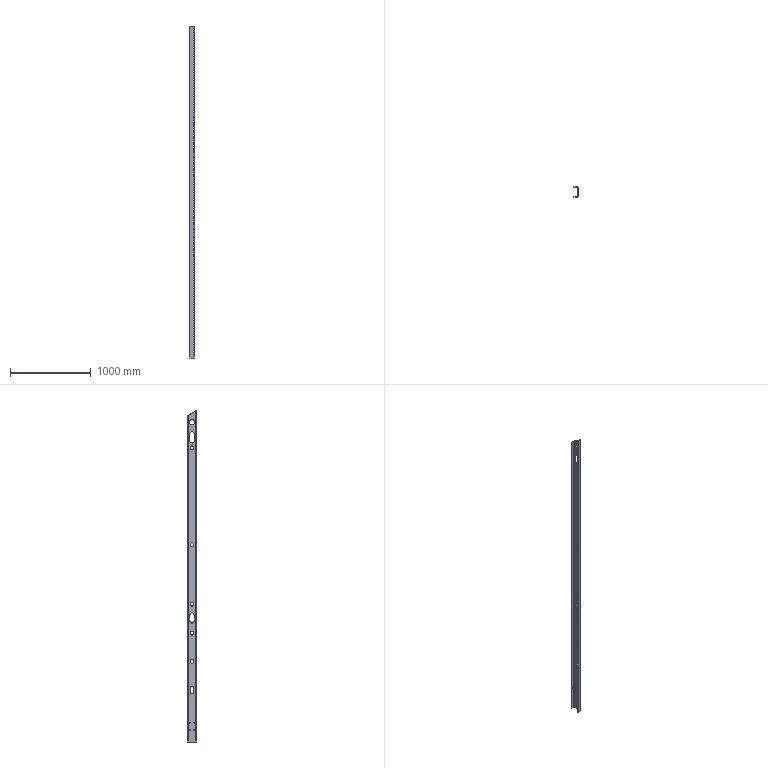Part | SolidWorks | features ICE 5, Cut 2, Extrusion 1 | 1 solid | 51 faces | box 50 x 120 x 4120 mm | volume 4129242 mm3 | cylinder 35 | plane 16 | commonest cylinder face diameters 50 x13 13 x8 20 x4 45 x3 60 x3 10 x2